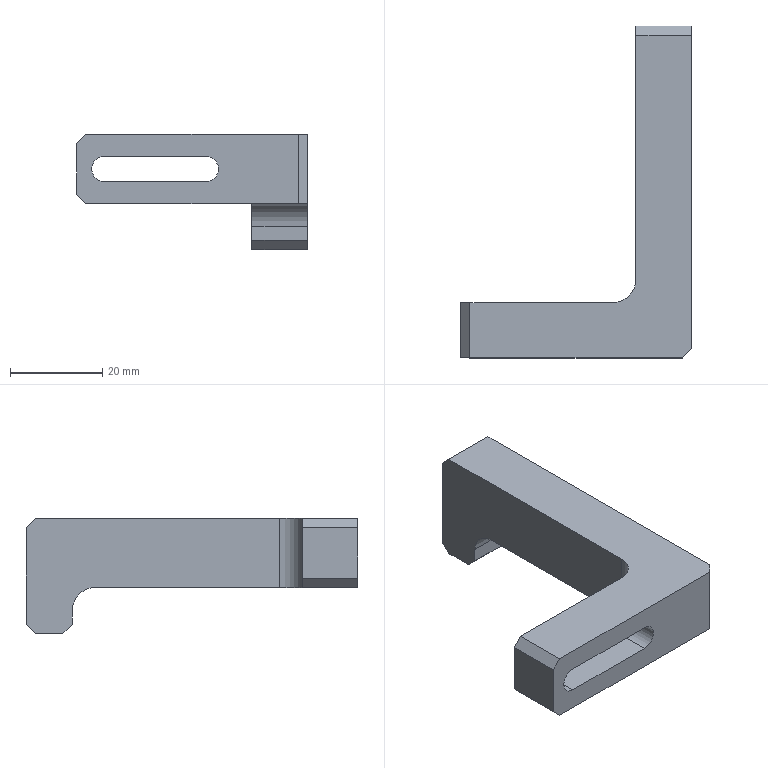NC program | NX | posted with a generic post | part box 50 x 72 x 25 mm
Lines 1 to 896 of 2700:
N10 G17 G21 G94 G90
(ADAPTIVE_MILLING , TOOL : D10)
N12 T15 M6
N14 G54
N16 G17 G0 G90 X24.031 Y-35.677 B0. C0. S9500 M3
N18 G43 Z30. H15
N20 Z-22.
N22 G94 G1 Z-25. F1000.
N24 X24.351 Y-34.954 F3500.
N26 X24.648 Y-34.221
N28 G3 X24.031 Y-33.031 R1.015
N30 X20.798 Y-32.59 R11.435
N32 X11.174 Y-32.505 R445.113
N34 G1 X-3.139 Y-32.504
N36 X-36.764
N38 X-36.951 Y-32.502
N40 X-37.076 Y-32.497
N42 X-37.201 Y-32.488
N44 G2 X-41.761 Y-29.352 R6.036
N46 X-43.27 Y-23.981 R12.881
N48 X-43.489 Y-15.799 R102.383
N50 G1 X-43.492 Y-13.487
N52 X-43.494 Y-7.737
N54 Y25.826
N56 X-43.492 Y25.951
N58 X-43.487 Y26.076
N60 X-43.483 Y26.138
N62 G2 X-40.394 Y30.727 R5.998
N64 X-35.032 Y32.263 R12.698
N66 X-26.913 Y32.488 R99.06
N68 G1 X-24.6 Y32.491
N70 X-19.6 Y32.493
N72 X36.837
N74 X36.962 Y32.491
N76 X37.087 Y32.486
N78 X37.15 Y32.482
N80 G2 X41.702 Y29.439 R5.988
N82 X43.266 Y24.022 R12.634
N84 X43.492 Y13.903 R126.694
N86 G1 X43.494 Y9.215
N88 Y-25.847
N90 X43.492 Y-25.972
N92 X43.486 Y-26.097
N94 X43.482 Y-26.16
N96 X43.471 Y-26.284
N98 G2 X40.269 Y-30.802 R6.081
N100 X34.762 Y-32.288 R13.252
N102 X25.143 Y-32.418 R86.065
N104 G3 X13.405 Y-32.016 R124.596
N106 G1 X11.092 Y-32.012
N108 X6.53 Y-32.01
N110 X-34.595 Y-32.009
N112 X-34.783 Y-32.007
N114 X-34.97 Y-32.001
N116 X-35.095 Y-31.995
N118 G2 X-41.15 Y-27.928 R7.445
N120 X-42.744 Y-21.931 R15.233
N122 X-42.985 Y-12.062 R124.05
N124 G1 X-42.988 Y-8.937
N126 X-42.989 Y2.376
N128 X-42.988 Y23.688
N130 X-42.987 Y23.813
N132 X-42.983 Y23.938
N134 X-42.977 Y24.063
N136 G2 X-38.883 Y30.165 R7.438
N138 X-32.758 Y31.758 R15.496
N140 X-22.888 Y31.984 R135.428
N142 G1 X-19.638 Y31.987
N144 X-6.513 Y31.988
N146 X34.675
N148 X34.8 Y31.986
N150 X34.925 Y31.983
N152 X35.112 Y31.974
N154 G2 X41.16 Y27.897 R7.442
N156 X42.741 Y21.96 R15.246
N158 X42.984 Y12.466 R120.578
N160 G1 X42.987 Y9.716
N162 X42.989 Y2.778
N164 Y-23.659
N166 X42.987 Y-23.784
N168 X42.982 Y-23.972
N170 X42.976 Y-24.096
N172 G2 X38.798 Y-30.21 R7.465
N174 X32.786 Y-31.756 R15.655
N176 X22.609 Y-31.72 R67.368
N178 G3 X8.737 Y-31.517 R304.425
N180 G1 X2.612 Y-31.515
N182 X-32.325
N184 X-32.888 Y-31.511
N186 X-33.075 Y-31.508
N188 X-33.325 Y-31.499
N190 X-33.512 Y-31.489
N192 G2 X-40.707 Y-26.527 R8.464
N194 X-42.241 Y-20.186 R17.685
N196 X-42.48 Y-9.253 R152.102
N198 G1 X-42.483 Y-5.566
N200 Y16.434
N202 Y21.747
N204 X-42.481 Y21.997
N206 X-42.477 Y22.184
N208 X-42.473 Y22.309
N210 G2 X-40.396 Y27.577 R8.169
N212 X-37.245 Y30.018 R5.845
N214 X-30.396 Y31.311 R22.269
N216 X-19.086 Y31.48 R233.51
N218 G1 X-13.773 Y31.482
N220 X32.789
N222 X33.039 Y31.48
N224 X33.289 Y31.472
N226 X33.414 Y31.467
N228 X33.539 Y31.46
N230 G2 X40.665 Y26.594 R8.422
N232 X42.239 Y20.2 R17.479
N234 X42.478 Y10.268 R135.88
N236 G1 X42.482 Y7.393
N238 X42.483 Y0.456
N240 Y-21.794
N242 X42.48 Y-22.044
N244 X42.473 Y-22.294
N246 X42.467 Y-22.419
N248 G2 X40.396 Y-27.577 R8.165
N250 X37.187 Y-30.04 R5.882
N252 X30.084 Y-31.329 R22.993
N254 X23.337 Y-31.241 R73.285
N256 G3 X7.902 Y-31.023 R375.345
N258 G1 X2.34 Y-31.021
N260 X-30.223 Y-31.02
N262 X-31.098 Y-31.015
N264 X-31.41 Y-31.012
N266 X-31.66 Y-31.006
N268 X-31.848 Y-31.
N270 G2 X-40.25 Y-25.296 R9.263
N272 X-41.747 Y-18.559 R19.97
N274 X-41.976 Y-5.626 R204.551
N276 G1 X-41.978 Y0.624
N278 Y20.062
N280 X-41.976 Y20.374
N282 X-41.971 Y20.624
N284 X-41.964 Y20.874
N286 X-41.952 Y21.124
N288 G2 X-41.116 Y24.76 R11.452
N290 G1 X-41.106 Y24.822
N292 X-41.1 Y24.884
N294 Y24.966
N296 X-41.096 Y25.033
N298 X-40.931 Y26.287
N300 X-40.924 Y26.319
N302 X-40.913 Y26.351
N304 X-40.43 Y27.519
N306 X-40.415 Y27.549
N308 X-39.579 Y28.627
N310 X-38.549 Y29.415
N312 G2 X-36.109 Y30.086 R5.764
N314 X-24.405 Y30.946 R70.892
N316 G1 X-23.28 Y30.956
N318 X-21.905 Y30.964
N320 X-20.092 Y30.971
N322 X-17.467 Y30.975
N324 X-12.342 Y30.977
N326 X31.095
N328 G2 X37.456 Y28.983 R9.555
N330 X39.423 Y26.79 R10.238
N332 X41.073 Y23.712 R5.843
N334 X41.911 Y15.206 R42.593
N336 X41.978 Y-3.043 R902.168
N338 G1 Y-20.106
N340 X41.975 Y-20.418
N342 X41.972 Y-20.606
N344 X41.964 Y-20.856
N346 X41.956 Y-21.043
N348 G2 X41.119 Y-24.742 R11.025
N350 G1 X41.109 Y-24.803
N352 X41.101 Y-24.865
N354 X41.1 Y-24.88
N356 Y-24.966
N358 X41.096 Y-25.033
N360 X40.931 Y-26.287
N362 X40.924 Y-26.319
N364 X40.913 Y-26.351
N366 X40.43 Y-27.519
N368 X40.415 Y-27.549
N370 G3 X42.129 Y-28.567 R1.
N372 G1 X42.207 Y-28.456
N374 X43.359 Y-26.821 Z-24.9
N376 X43.796 Y-26.205
N378 X44.22 Y-25.579
N380 X44.312 Y-25.299
N382 X44.598 Y-23.638
N384 X44.842 Y-21.971
N386 X44.946 Y-20.854
N388 X45.014 Y-19.733
N390 X45.362 Y-10.366
N392 G3 X45.154 Y12.103 R243.763
N394 G1 X44.632 Y21.466
N396 G3 X43.503 Y26.088 R12.911
N398 X42.092 Y28.325 R10.947
N400 G1 X40.973 Y29.694
N402 X39.84 Y31.051
N404 G3 X37.364 Y32.811 R7.906
N406 X33.532 Y33.79 R10.235
N408 X27.294 Y33.983 R113.382
N410 G1 X-33.859
N412 G3 X-34.484 Y33.763 R1.039
N414 G1 X-35.913 Y32.62
N416 X-36.452 Y32.193 Z-24.934
N418 X-36.978 Y31.751 Z-24.969
N420 G3 X-37.233 Y31.192 Z-25. R1.045
N422 X-36.109 Y30.086 R1.003
N424 X-27.847 Y30.361 R195.35
N426 G2 X-7.473 Y30.472 R883.198
N428 G1 X29.59
N430 X29.902 Y30.469
N432 X30.277 Y30.463
N434 X30.527 Y30.456
N436 X30.777 Y30.446
N438 G2 X33.273 Y30.1 R16.161
N440 X35.351 Y29.913 R10.409
N442 X37.63 Y28.582 R5.911
N444 G1 X39.442 Y26.77
N446 G3 X41.149 Y27.498 R1.001
N448 X40.934 Y28.165 Z-24.965 R1.678
N450 G1 X40.395 Y29.341 Z-24.9
N452 X39.588 Y31.085
N454 X39.442 Y31.27
N456 X38.819 Y31.877
N458 G3 X37.96 Y32.334 R2.596
N460 X34.932 Y32.995 R14.741
N462 X29.331 Y33.441 R85.852
N464 G1 X28.084 Y33.471
N466 X26.836 Y33.486
N468 X-26.686 Y33.36
N470 X-28.735 Y33.332
N472 X-30.784 Y33.282
N474 X-30.945 Y33.26
N476 X-31.102 Y33.221
N478 X-32.774 Y32.605
N480 X-34.422 Y31.99 Z-24.988
N482 X-34.621 Y31.856 Z-25.
N484 G3 X-33.966 Y30.1 R1.001
N486 G1 X33.284
N488 X34.033 Y30.096
N490 X35.351 Y29.913
N492 X36.577 Y29.396
N494 X37.63 Y28.582
N496 X39.627 Y26.579
N498 X40.43 Y25.519
N500 X40.924 Y24.319
N502 G2 X41.124 Y21.467 R16.402
N504 X41.468 Y6.598 R238.541
N506 G1 X41.471 Y2.911
N508 X41.473 Y-7.652
N510 X41.472 Y-18.589
N512 X41.47 Y-18.902
N514 X41.464 Y-19.277
N516 X41.457 Y-19.527
N518 G2 X41.1 Y-22.386 R18.888
N520 G1 Y-24.886
N522 G3 X42.202 Y-25.984 R1.1
N524 X43.3 Y-24.886 R1.1
N526 G1 Y22.216
N528 G3 X42.198 Y23.314 R1.1
N530 X41.1 Y22.216 R1.1
N532 G1 Y-22.409
N534 X41.096 Y-25.033
N536 X40.913 Y-26.351
N538 X40.396 Y-27.577
N540 X39.579 Y-28.627
N542 X38.549 Y-29.415
N544 G2 X36.109 Y-30.086 R5.764
N546 X24.278 Y-30.757 R53.632
N548 G3 X1.905 Y-30.526 R633.402
N550 G1 X-28.032 Y-30.525
N552 X-29.595 Y-30.517
N554 X-30.032 Y-30.512
N556 X-30.282 Y-30.506
N558 G2 X-37.515 Y-27.63 R9.983
N560 X-40.688 Y-21.287 R12.799
N562 X-41.408 Y-13.395 R42.412
N564 X-41.473 Y3.98 R870.081
N566 X-41.433 Y20.042 R813.793
N568 X-41.1 Y22.391 R26.785
N570 G1 Y24.891
N572 G3 X-42.842 Y25.562 R1.001
N574 X-43.137 Y24.967 Z-24.967 R1.691
N576 G1 X-43.593 Y23.717 Z-24.9
N578 X-43.937 Y22.789
N580 X-44.263 Y21.853
N582 X-44.282 Y21.709
N584 X-44.486 Y18.343
N586 X-44.643 Y14.975
N588 X-44.686 Y12.728
N590 X-44.689 Y10.48
N592 X-44.401 Y-15.146
N594 G3 X-43.755 Y-21.335 R34.001
N596 G1 X-43.279 Y-23.659
N598 G3 X-41.587 Y-27.239 R11.046
N600 G1 X-40.564 Y-28.602
N602 X-39.519 Y-29.947
N604 G3 X-37.955 Y-31.263 R6.717
N606 X-34.809 Y-32.741 R15.776
N608 X-32.748 Y-33.19 R13.647
N610 X-29.033 Y-33.509 R24.608
N612 G1 X33.859 Y-33.983
N614 G3 X34.493 Y-33.762 R1.039
N616 G1 X36.127 Y-32.45
N618 X36.976 Y-31.754 Z-24.955
N620 G3 X37.227 Y-30.919 Z-25. R1.016
N622 X36.109 Y-30.086 R1.005
N624 X28.595 Y-30.285 R302.572
N626 G2 X16.034 Y-30.076 R943.331
N628 G1 X14.597 Y-30.062
N630 X13.097 Y-30.052
N632 X11.16 Y-30.044
N634 X8.722 Y-30.037
N636 X5.285 Y-30.033
N638 X-1.403 Y-30.031
N640 X-25.84
N642 X-28.215 Y-30.019
N644 X-28.715 Y-30.013
N646 X-29.028 Y-30.006
N648 G2 X-35.52 Y-28.105 R11.186
N650 X-39.814 Y-21.68 R11.769
N652 X-40.844 Y-14.018 R31.965
N654 X-40.966 Y-1.02 R449.524
N656 G1 X-40.967 Y8.543
N658 X-40.968 Y11.98
N660 X-40.969 Y12.006
N662 X-41.096 Y12.967
N664 X-41.1 Y13.034
N666 Y22.409
N668 G3 X-42.823 Y23.099 R1.001
N670 X-43.141 Y22.477 Z-24.965 R1.685
N672 G1 X-43.592 Y21.263 Z-24.9
N674 X-44.254 Y19.462
N676 X-44.282 Y19.227
N678 Y-10.148
N680 G3 X-43.499 Y-18.828 R48.938
N682 G1 X-43.168 Y-20.672
N684 X-42.814 Y-22.512
N686 G3 X-41.13 Y-26.512 R12.824
N688 X-38.348 Y-29.827 R13.587
N690 X-31.623 Y-32.781 R13.087
N692 X-27.897 Y-33.095 R41.046
N694 X-15.715 Y-33.411 R385.067
N696 G1 X-12.904 Y-33.416
N698 X30.901 Y-33.275
N700 X31.129 Y-33.22
N702 X33.114 Y-32.483
N704 X34.445 Y-31.978 Z-24.971
N706 G3 X34.846 Y-31.576 Z-25. R1.053
N708 X33.966 Y-30.1 R1.002
N710 G1 X24.034
N712 X23.967 Y-30.096
N714 G3 X15.601 Y-29.588 R58.
N716 G1 X14.476 Y-29.575
N718 X13.163 Y-29.564
N720 X11.538 Y-29.554
N722 X9.538 Y-29.547
N724 X6.851 Y-29.541
N726 X2.726 Y-29.538
N728 X-7.961 Y-29.536
N730 X-23.649
N732 X-26.899 Y-29.52
N734 X-27.399 Y-29.514
N736 G2 X-33.25 Y-28.424 R13.813
N738 X-38.878 Y-22.018 R11.189
N740 X-40.251 Y-14.547 R25.799
N742 X-40.459 Y-1.613 R244.174
N744 G1 X-40.461 Y3.512
N746 X-40.462 Y9.825
N748 X-40.465 Y10.262
N750 X-40.467 Y10.387
N752 X-40.47 Y10.45
N754 X-40.478 Y10.512
N756 X-40.488 Y10.573
N758 X-40.502 Y10.634
N760 X-40.522 Y10.705
N762 X-40.913 Y11.649
N764 X-40.924 Y11.681
N766 X-40.931 Y11.713
N768 X-40.971 Y12.023
N770 G3 X-42.372 Y12.805 R1.003
N772 X-42.963 Y12.081 Z-24.952 R1.135
N774 G1 X-43.339 Y11.117 Z-24.9
N776 X-44.123 Y9.087
N778 X-44.153 Y8.841
N780 Y-6.159
N782 G3 X-43.331 Y-16.091 R60.929
N784 G1 X-43.015 Y-18.001
N786 X-42.68 Y-19.908
N788 G3 X-40.846 Y-25.06 R20.824
N790 X-39.109 Y-27.644 R16.46
N792 G1 X-38.04 Y-28.921
N794 G3 X-36.436 Y-30.187 R6.913
N796 X-33.756 Y-31.51 R25.714
N798 X-31.231 Y-32.143 R11.555
N800 X-27.517 Y-32.48 R25.013
N802 G1 X19.532 Y-33.113
N804 X19.728 Y-33.092
N806 X19.92 Y-33.04
N808 X21.801 Y-32.28
N810 X22.425 Y-32.033 Z-24.934
N812 X23.04 Y-31.765 Z-24.967
N814 G3 X23.453 Y-31.268 Z-25. R1.041
N816 X22.713 Y-29.931 R1.004
N818 X19.1 Y-29.261 R11.602
N820 X5.166 Y-29.046 R256.197
N822 G1 X0.479 Y-29.043
N824 X-16.646 Y-29.042
N826 X-21.459 Y-29.041
N828 X-25.646 Y-29.021
N830 X-26.271 Y-29.013
N832 G2 X-32.092 Y-28.054 R15.346
N834 X-38.217 Y-21.546 R11.348
N836 X-39.716 Y-13.911 R25.326
N838 X-39.953 Y-0.915 R222.499
N840 G3 X-39.996 Y9.459 R528.027
N842 X-40.43 Y10.481 R1.625
N844 G1 X-40.525 Y10.712
N846 G3 X-41.69 Y11.3 R1.005
N848 X-42.402 Y10.649 Z-24.95 R1.037
N850 G1 X-42.81 Y9.741 Z-24.9
N852 X-43.247 Y8.778
N854 X-43.668 Y7.808
N856 X-43.707 Y7.53
N858 Y-2.47
N860 G3 X-42.757 Y-14.897 R82.407
N862 G1 X-42.381 Y-17.367
N864 X-41.985 Y-19.834
N866 G3 X-39.912 Y-24.989 R14.309
N868 G1 X-39.552 Y-25.494
N870 X-39.175 Y-25.987
N872 X-38.061 Y-27.357
N874 X-36.934 Y-28.714
N876 G3 X-34.464 Y-30.48 R7.756
N878 X-32.47 Y-31.172 R12.464
N880 X-28.803 Y-31.798 R17.271
N882 X-21.316 Y-32.124 R190.312
N884 G1 X19.236 Y-33.
N886 X19.457 Y-32.976
N888 X19.67 Y-32.911
N890 X21.411 Y-32.122
N892 X22.01 Y-31.857 Z-24.933
N894 X22.598 Y-31.568 Z-24.966
N896 G3 X22.995 Y-31.022 Z-25. R1.038
N898 X22.418 Y-29.818 R1.005
N900 X17.863 Y-28.782 R12.036
N902 X6.055 Y-28.554 R195.202
N904 G1 X2.805 Y-28.55
N906 X-3.257 Y-28.548
N908 X-19.257 Y-28.547
N910 X-24.57 Y-28.521
N912 G2 X-30.326 Y-27.881 R20.186
N914 X-37.528 Y-21.16 R11.426
N916 X-39.163 Y-13.555 R24.459
N918 X-39.446 Y-0.374 R194.145
N920 G3 X-39.511 Y8.563 R249.756
N922 X-40.184 Y10.146 R2.257
N924 X-41.226 Y10.506 R1.01
N926 X-41.903 Y9.926 Z-24.954 R1.049
N928 G1 X-42.416 Y8.977 Z-24.9
N930 X-43.246 Y7.439
N932 X-43.332 Y7.208
N934 X-43.365 Y6.964
N936 X-43.368 Y3.349
N938 X-43.352 Y-0.266
N940 G3 X-42.708 Y-9.872 R97.495
N942 G1 X-41.943 Y-16.283
N944 G3 X-40.515 Y-22.128 R30.77
N946 X-37.878 Y-26.511 R13.627
N948 X-33.214 Y-30.016 R17.246
N950 X-29.984 Y-31.045 R12.435
N952 X-27.014 Y-31.36 R19.914
N954 G1 X18.299 Y-32.612
N956 X18.532 Y-32.587
N958 X18.755 Y-32.516
N960 X20.438 Y-31.718
N962 X21.032 Y-31.442 Z-24.933
N964 X21.616 Y-31.143 Z-24.966
N966 G3 X22.003 Y-30.59 Z-25. R1.038
N968 X21.481 Y-29.43 R1.007
N970 X18.773 Y-28.526 R6.475
N972 X11.104 Y-28.096 R58.572
N974 G1 X10.042 Y-28.084
N976 X8.792 Y-28.074
N978 X7.167 Y-28.066
N980 X5.042 Y-28.06
N982 X1.917 Y-28.056
N984 X-3.833 Y-28.053
N986 X-17.083 Y-28.052
N988 X-23.396 Y-28.021
N990 G2 X-29.166 Y-27.473 R23.143
N992 X-36.974 Y-20.476 R11.681
N994 X-38.64 Y-12.815 R24.652
N996 X-38.937 Y-0.821 R168.33
N998 G3 X-39.035 Y7.864 R162.602
N1000 X-39.488 Y9.303 R2.308
N1002 G1 X-39.579 Y9.373
N1004 X-39.605 Y9.395
N1006 X-39.627 Y9.421
N1008 X-39.779 Y9.619
N1010 G3 X-41.077 Y9.874 R1.005
N1012 X-41.577 Y9.049 Z-24.95 R1.037
N1014 G1 X-41.714 Y8.062 Z-24.9
N1016 X-41.88 Y6.893
N1018 X-42.029 Y5.722
N1020 Y-8.653
N1022 G3 X-41.173 Y-17.121 R43.211
N1024 X-40.265 Y-20.315 R27.159
N1026 G1 X-39.891 Y-21.374
N1028 X-39.476 Y-22.417
N1030 G3 X-37.301 Y-25.744 R13.923
N1032 G1 X-36.142 Y-27.051
N1034 G3 X-32.887 Y-29.307 R10.968
N1036 X-30.091 Y-30.348 R18.668
N1038 X-27.335 Y-30.81 R17.259
N1040 G1 X-25.936 Y-30.915
N1042 X-24.534 Y-30.969
N1044 X17.477 Y-31.608
N1046 X17.63 Y-31.599
N1048 X19.781 Y-31.298
N1050 X20.428 Y-31.214 Z-24.933
N1052 X21.072 Y-31.103 Z-24.965
N1054 G3 X21.609 Y-30.687 Z-25. R1.038
N1056 X21.374 Y-29.358 R1.005
N1058 X18.405 Y-28.137 R6.03
N1060 X10.994 Y-27.617 R47.935
N1062 X-3.881 Y-27.559 R798.925
N1064 G2 X-24.693 Y-27.469 R942.758
N1066 X-31.505 Y-25.665 R14.046
N1068 X-36.864 Y-18.667 R12.784
N1070 X-38.209 Y-10.869 R29.809
N1072 X-38.442 Y3.002 R271.273
N1074 G3 X-38.646 Y7.868 R34.553
N1076 X-39.506 Y9.317 R1.848
N1078 X-40.607 Y9.393 R1.01
N1080 X-41.113 Y8.632 Z-24.953 R1.045
N1082 G1 X-41.326 Y7.601 Z-24.9
N1084 X-41.75 Y5.521
N1086 X-41.756 Y-5.206
N1088 G3 X-41.036 Y-13.896 R53.484
N1090 G1 X-40.49 Y-17.098
N1092 G3 X-38.993 Y-21.71 R20.352
N1094 X-36.178 Y-25.777 R14.489
N1096 X-32.273 Y-28.696 R18.842
N1098 X-29.29 Y-29.77 R10.929
N1100 X-23.736 Y-30.435 R29.642
N1102 G1 X17.08 Y-31.304
N1104 X17.24 Y-31.294
N1106 X19.38 Y-30.995
N1108 X20.029 Y-30.91 Z-24.933
N1110 X20.675 Y-30.799 Z-24.966
N1112 G3 X21.21 Y-30.386 Z-25. R1.038
N1114 X20.977 Y-29.054 R1.005
N1116 X17.738 Y-27.681 R6.529
N1118 X9.892 Y-27.123 R49.504
N1120 X-4.858 Y-27.064 R794.494
N1122 G2 X-24.044 Y-26.955 R700.724
N1124 X-30.906 Y-25.091 R14.275
N1126 X-36.267 Y-18.163 R12.985
N1128 X-37.711 Y-9.815 R30.345
N1130 X-37.951 Y3.744 R308.588
N1132 G3 X-38.309 Y7.905 R17.713
N1134 X-39.191 Y9.075 R1.808
N1136 X-40.31 Y9.142 R1.01
N1138 X-40.799 Y8.389 Z-24.954 R1.048
N1140 G1 X-41.015 Y7.34 Z-24.9
N1142 X-41.436 Y5.28
N1144 X-41.446 Y0.231
N1146 X-41.427 Y-4.818
N1148 G3 X-40.547 Y-13.491 R56.113
N1150 G1 X-39.865 Y-17.176
N1152 G3 X-37.709 Y-22.305 R15.172
N1154 G1 X-37.348 Y-22.81
N1156 X-36.971 Y-23.304
N1158 X-34.215 Y-26.692
N1160 X-33.633 Y-27.339
N1162 G3 X-32.801 Y-27.843 R2.573
N1164 G1 X-29.744 Y-28.932
N1166 G3 X-24.612 Y-29.891 R22.756
N1168 G1 X-23.118 Y-29.968
N1170 X16.584 Y-30.923
N1172 X16.747 Y-30.914
N1174 X18.879 Y-30.615
N1176 X19.531 Y-30.53 Z-24.933
N1178 X20.178 Y-30.419 Z-24.966
N1180 G3 X20.712 Y-30.01 Z-25. R1.039
N1182 X20.481 Y-28.673 R1.005
N1184 X17.924 Y-27.403 R5.205
N1186 X11.038 Y-26.68 R33.863
N1188 X-11.336 Y-26.565 R982.532
N1190 G2 X-23.647 Y-26.426 R309.843
N1192 X-30.782 Y-24.219 R13.944
N1194 X-35.858 Y-17.135 R13.488
N1196 X-37.214 Y-8.769 R32.47
N1198 X-37.457 Y3.477 R329.353
N1200 G3 X-37.913 Y7.689 R15.939
N1202 X-38.775 Y8.756 R1.774
N1204 X-39.891 Y8.825 R1.01
N1206 X-40.383 Y8.07 Z-24.953 R1.047
N1208 G1 X-40.599 Y7.025 Z-24.9
N1210 X-41.02 Y4.961
N1212 X-41.025 Y1.697
N1214 X-41.011 Y-1.567
N1216 G3 X-40.318 Y-10.091 R71.458
N1218 G1 X-39.959 Y-12.627
N1220 X-39.58 Y-15.16
N1222 G3 X-38.164 Y-19.795 R19.55
N1224 X-35.905 Y-23.503 R20.693
N1226 X-32.434 Y-26.774 R17.485
N1228 X-29.509 Y-28.218 R12.328
N1230 X-25.293 Y-29.235 R16.464
N1232 G1 X-24.673 Y-29.277
N1234 X-13.433 Y-29.768
N1236 X-8.438 Y-29.969
N1238 X-3.443 Y-30.144
N1240 X16.596 Y-30.826
N1242 X18.638 Y-30.407
N1244 X19.293 Y-30.275 Z-24.933
N1246 X19.943 Y-30.12 Z-24.967
N1248 G3 X20.439 Y-29.699 Z-25. R1.041
N1250 X20.373 Y-28.579 R1.01
N1252 X18.378 Y-27.25 R3.898
N1254 X12.725 Y-26.306 R21.555
N1256 X-2.334 Y-26.077 R288.211
N1258 G2 X-22.146 Y-25.962 R879.934
N1260 X-28.859 Y-24.444 R16.124
N1262 X-35.04 Y-17.278 R13.018
N1264 X-36.633 Y-9.087 R28.624
N1266 X-36.946 Y2.47 R222.466
N1268 G3 X-37.417 Y7.184 R19.682
N1270 X-38.244 Y8.457 R1.919
N1272 G1 X-38.519 Y8.57
N1274 G3 X-39.41 Y8.508 R1.015
N1276 X-39.915 Y7.742 Z-24.953 R1.146
N1278 G1 X-40.211 Y6.73 Z-24.9
N1280 X-40.493 Y5.775
N1282 X-40.759 Y4.815
N1284 X-40.769 Y4.673
N1286 X-40.757 Y0.508
N1288 G3 X-40.356 Y-4.674 R48.529
N1290 G1 X-39.034 Y-14.587
N1292 G3 X-37.294 Y-19.876 R15.696
N1294 G1 X-36.832 Y-20.687
N1296 X-36.335 Y-21.478
N1298 X-35.07 Y-23.333
N1300 G3 X-31.061 Y-26.815 R12.07
N1302 G1 X-30.384 Y-27.126
N1304 X-29.686 Y-27.389
N1306 X-27.318 Y-28.154
N1308 G3 X-24.272 Y-28.761 R18.727
N1310 G1 X-22.408 Y-28.932
N1312 X-20.539 Y-29.048
N1314 X16.324 Y-30.631
N1316 X16.572 Y-30.611
N1318 X18.466 Y-30.213
N1320 X19.13 Y-30.079 Z-24.934
N1322 X19.788 Y-29.923 Z-24.968
N1324 G3 X20.277 Y-29.518 Z-25. R1.042
N1326 X20.221 Y-28.381 R1.01
N1328 X17.949 Y-26.812 R4.283
N1330 X11.988 Y-25.816 R22.614
N1332 X-0.759 Y-25.586 R243.861
N1334 G2 X-21.507 Y-25.452 R809.147
N1336 X-28.385 Y-23.832 R16.181
N1338 X-34.496 Y-16.672 R13.209
N1340 X-36.116 Y-8.423 R28.856
N1342 X-36.459 Y2.507 R257.165
N1344 G3 X-37.021 Y7.021 R17.159
N1346 X-37.876 Y8.304 R2.091
N1348 G1 X-38.28 Y8.471
N1350 G3 X-39.224 Y8.375 R1.014
N1352 X-39.674 Y7.658 Z-24.957 R1.164
N1354 G1 X-40.003 Y6.575 Z-24.9
N1356 X-40.522 Y4.836
N1358 X-40.53 Y4.574
N1360 X-39.037 Y-10.351
N1362 G3 X-37.605 Y-17.046 R31.739
N1364 X-35.881 Y-20.625 R19.458
N1366 X-33.977 Y-23.396 R30.465
N1368 X-31.348 Y-25.655 R10.355
N1370 X-27.635 Y-27.379 R19.31
N1372 X-22.749 Y-28.27 R19.771
N1374 G1 X-7.982 Y-29.085
N1376 X-1.326 Y-29.432
N1378 X16.058 Y-30.284
N1380 X16.312 Y-30.264
N1382 X18.193 Y-29.868
N1384 X18.859 Y-29.733 Z-24.934
N1386 X19.52 Y-29.576 Z-24.968
N1388 G3 X20.007 Y-29.177 Z-25. R1.043
N1390 X19.955 Y-28.034 R1.01
N1392 X17.644 Y-26.408 R4.469
N1394 X11.632 Y-25.348 R22.421
N1396 X-0.926 Y-25.094 R219.593
N1398 G2 X-20.425 Y-24.965 R900.963
N1400 X-27.292 Y-23.536 R17.564
N1402 X-33.904 Y-16.198 R13.227
N1404 X-35.591 Y-7.9 R28.524
N1406 X-35.975 Y2.467 R295.247
N1408 G3 X-36.655 Y6.961 R15.487
N1410 X-37.469 Y8.136 R2.149
N1412 G1 X-37.931 Y8.327
N1414 G3 X-39.031 Y8.1 R1.01
N1416 X-39.305 Y7.241 Z-24.953 R1.047
N1418 G1 X-39.236 Y6.177 Z-24.9
N1420 X-39.096 Y3.98
N1422 X-39.101 Y-0.304
N1424 X-39.082 Y-4.588
N1426 G3 X-38.425 Y-10.959 R42.25
N1428 X-37.428 Y-15.422 R38.228
N1430 X-36.229 Y-18.741 R29.672
N1432 X-33.445 Y-22.826 R13.957
N1434 G1 X-32.992 Y-23.25
N1436 X-32.525 Y-23.658
N1438 X-30.683 Y-25.154
N1440 G3 X-26.653 Y-27.047 R11.379
N1442 X-22.359 Y-27.756 R21.622
N1444 G1 X15.791 Y-29.937
N1446 X16.055 Y-29.917
N1448 X17.924 Y-29.523
N1450 X18.591 Y-29.386 Z-24.934
N1452 X19.254 Y-29.229 Z-24.968
N1454 G3 X19.739 Y-28.832 Z-25. R1.043
N1456 X19.688 Y-27.687 R1.01
N1458 X17.625 Y-26.11 R4.103
N1460 X11.893 Y-24.931 R19.649
N1462 X-0.037 Y-24.605 R162.606
N1464 G1 X-1.912 Y-24.599
N1466 X-2.662 Y-24.596
N1468 X-3.662 Y-24.594
N1470 X-4.162 Y-24.592
N1472 X-4.412 Y-24.591
N1474 X-4.975 Y-24.588
N1476 X-5.475 Y-24.586
N1478 X-5.912 Y-24.585
N1480 X-6.662 Y-24.583
N1482 X-7.037 Y-24.581
N1484 X-7.537 Y-24.58
N1486 X-7.787 Y-24.579
N1488 X-8.287 Y-24.578
N1490 X-8.975 Y-24.576
N1492 X-9.912 Y-24.571
N1494 X-10.475 Y-24.569
N1496 X-11.1 Y-24.568
N1498 X-11.725 Y-24.564
N1500 X-13.225 Y-24.559
N1502 X-14.287 Y-24.555
N1504 G2 X-22.028 Y-24.28 R76.229
N1506 X-30.644 Y-20.066 R13.362
N1508 X-34.346 Y-12.382 R16.748
N1510 X-35.286 Y-3.319 R49.548
N1512 G3 X-35.697 Y4.542 R88.065
N1514 X-36.712 Y7.663 R7.143
N1516 X-37.524 Y8.158 R1.617
N1518 X-38.622 Y7.934 R1.01
N1520 X-38.899 Y7.074 Z-24.953 R1.047
N1522 G1 X-38.83 Y6.012 Z-24.9
N1524 X-38.689 Y3.812
N1526 X-38.576 Y-1.431
N1528 G3 X-38.124 Y-7.403 R82.501
N1530 G1 X-37.844 Y-9.887
N1532 X-37.545 Y-12.369
N1534 G3 X-36.495 Y-16.073 R16.352
N1536 X-35.219 Y-18.78 R27.4
N1538 G1 X-34.667 Y-19.796
N1540 X-34.073 Y-20.788
N1542 G3 X-31.913 Y-23.248 R13.443
N1544 X-27.718 Y-25.875 R12.535
N1546 X-22.911 Y-27.1 R18.411
N1548 X-17.942 Y-27.533 R49.427
N1550 G1 X15.253 Y-28.685
N1552 X17.418 Y-28.824
N1554 X18.083 Y-28.872 Z-24.933
N1556 X18.749 Y-28.896 Z-24.967
N1558 G3 X19.342 Y-28.62 Z-25. R1.04
N1560 X19.57 Y-27.519 R1.01
N1562 X17.977 Y-25.998 R3.194
N1564 X12.691 Y-24.588 R15.514
N1566 X2.456 Y-24.132 R98.765
N1568 G1 X1.081 Y-24.121
N1570 X0.206 Y-24.116
N1572 X-0.231 Y-24.112
N1574 X-2.356 Y-24.103
N1576 X-3.794 Y-24.097
N1578 X-10.544 Y-24.07
N1580 X-14.169 Y-24.053
N1582 X-14.606 Y-24.05
N1584 X-15.044 Y-24.046
N1586 G2 X-22.275 Y-23.637 R48.165
N1588 X-32.664 Y-15.408 R13.29
N1590 X-34.535 Y-6.899 R27.537
N1592 X-35.01 Y2.213 R529.995
N1594 G3 X-35.874 Y6.736 R14.532
N1596 X-36.923 Y8. R2.147
N1598 G1 X-36.983 Y8.019
N1600 X-37.043 Y8.035
N1602 X-37.054 Y8.039
N1604 X-37.287 Y8.069
N1606 G3 X-38.135 Y7.774 R1.015
N1608 X-38.419 Y6.897 Z-24.953 R1.143
N1610 G1 X-38.43 Y5.848 Z-24.9
N1612 X-38.451 Y3.036
N1614 X-38.437 Y0.225
N1616 G3 X-38.098 Y-3.752 R36.644
N1618 G1 X-37.484 Y-8.083
N1620 X-36.85 Y-12.41
N1622 G3 X-35.294 Y-17.119 R16.652
N1624 G1 X-34.832 Y-17.928
N1626 X-34.323 Y-18.709
N1628 X-32.57 Y-21.171
N1630 G3 X-28.244 Y-24.781 R13.513
N1632 X-23.563 Y-26.377 R15.628
N1634 X-17.991 Y-27.015 R42.411
N1636 G1 X15.171 Y-28.511
N1638 X17.331 Y-28.65
N1640 X18.002 Y-28.698 Z-24.934
N1642 X18.674 Y-28.723 Z-24.967
N1644 G3 X19.259 Y-28.457 Z-25. R1.041
N1646 X19.499 Y-27.346 R1.01
N1648 X17.776 Y-25.614 R3.384
N1650 X12.568 Y-24.154 R15.356
N1652 X2.836 Y-23.651 R87.057
N1654 G1 X1.399 Y-23.635
N1656 X-0.101 Y-23.622
N1658 X-1.726 Y-23.613
N1660 X-6.226 Y-23.593
N1662 X-6.538 Y-23.59
N1664 X-7.038 Y-23.588
N1666 X-7.413 Y-23.586
N1668 X-7.913 Y-23.583
N1670 X-9.038 Y-23.579
N1672 X-9.476 Y-23.576
N1674 X-10.413 Y-23.573
N1676 X-10.851 Y-23.569
N1678 X-11.726 Y-23.567
N1680 G2 X-20.219 Y-23.319 R102.803
N1682 X-28.1 Y-20.309 R14.464
N1684 X-32.875 Y-12.766 R15.152
N1686 X-34.193 Y-3.821 R38.509
N1688 G3 X-34.748 Y3.968 R88.922
N1690 X-35.942 Y7.421 R7.923
N1692 X-37.056 Y8.039 R1.357
N1694 X-37.945 Y7.699 R1.014
N1696 X-38.188 Y6.874 Z-24.956 R1.154
N1698 G1 X-38.202 Y5.757 Z-24.9
N1700 X-38.22 Y3.692
N1702 X-36.771 Y-9.352
N1704 G3 X-34.728 Y-16.507 R21.653
N1706 X-32.458 Y-20.224 R24.277
N1708 X-26.621 Y-24.742 R14.807
N1710 X-19.983 Y-26.288 R19.342
N1712 G1 X15.064 Y-28.28
N1714 X17.225 Y-28.419
N1716 X17.9 Y-28.467 Z-24.934
N1718 X18.576 Y-28.493 Z-24.968
N1720 G3 X19.156 Y-28.233 Z-25. R1.042
N1722 X19.403 Y-27.115 R1.01
N1724 X17.638 Y-25.255 R3.521
N1726 X12.329 Y-23.704 R15.273
N1728 X1.912 Y-23.154 R88.838
N1730 G1 X0.725 Y-23.14
N1732 X-0.713 Y-23.128
N1734 X-2.775 Y-23.115
N1736 X-4.15 Y-23.108
N1738 X-5.025 Y-23.103
N1740 X-5.837 Y-23.098
N1742 X-6.275 Y-23.095
N1744 X-9.587 Y-23.08
N1746 G2 X-19.145 Y-22.855 R145.143
N1748 X-26.771 Y-20.342 R15.38
N1750 X-32.191 Y-12.669 R14.72
N1752 X-33.606 Y-4.436 R34.354
N1754 G3 X-34.224 Y3.412 R117.198
N1756 X-35.488 Y7.237 R9.158
N1758 X-36.772 Y8.002 R1.511
N1760 X-37.697 Y7.618 R1.011
N1762 X-37.905 Y6.829 Z-24.958 R1.187
N1764 G1 X-37.92 Y5.664 Z-24.9
N1766 X-37.937 Y3.655
N1768 X-36.619 Y-6.888
N1770 G3 X-34.607 Y-14.981 R36.197
N1772 X-31.421 Y-20.294 R19.739
N1774 X-29.398 Y-22.319 R20.321
N1776 X-25.948 Y-24.27 R11.566
N1778 X-19.914 Y-25.738 R25.592
N1780 G1 X-18.984 Y-25.834
N1782 X-18.053 Y-25.91
N1784 X17.08 Y-28.072
N1786 X17.756 Y-28.12 Z-24.934
N1788 X18.432 Y-28.146 Z-24.968
N1790 G3 X19.011 Y-27.888 Z-25. R1.042